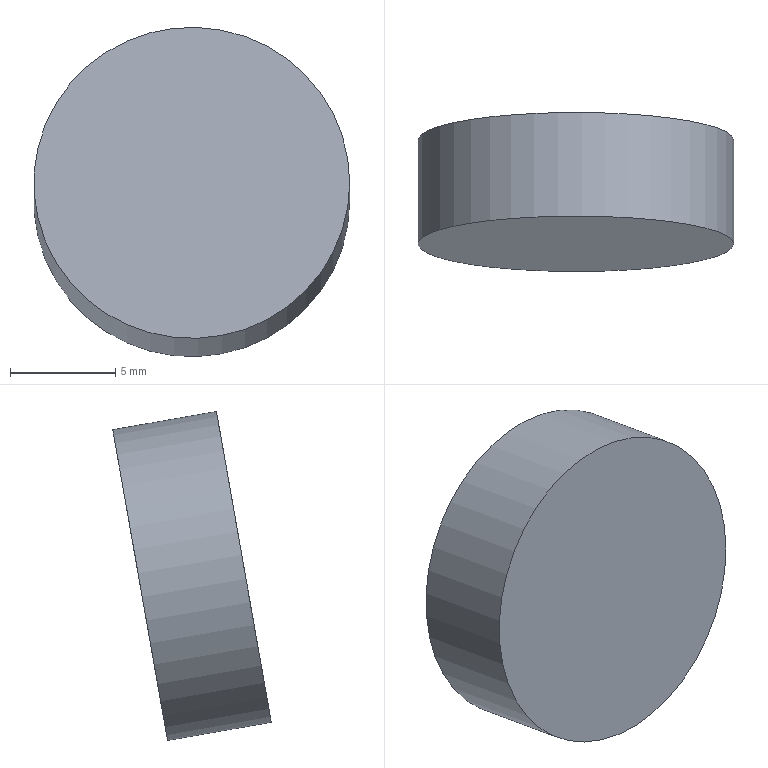Part | NX | features solid 2 | 1 solid | 3 faces | box 15 x 7.529 x 15.64 mm | volume 883.573 mm3 | plane 2 | cylinder 1 | commonest cylinder face diameters 15 x1
STEP:
#1=CARTESIAN_POINT('',(-1001.,-834.668,49.225));
#2=VERTEX_POINT('',#1);
#3=CARTESIAN_POINT('',(-1008.5,-834.668,49.225));
#4=DIRECTION('',(0.,-0.9848,0.1736));
#5=DIRECTION('',(1.,0.,0.));
#6=AXIS2_PLACEMENT_3D('',#3,#4,#5);
#7=CIRCLE('',#6,7.5);
#8=EDGE_CURVE('',#2,#2,#7,.T.);
#9=ORIENTED_EDGE('',*,*,#8,.T.);
#10=EDGE_LOOP('',(#9));
#11=FACE_BOUND('',#10,.T.);
#12=CARTESIAN_POINT('',(-1001.,-839.592,50.093));
#13=VERTEX_POINT('',#12);
#14=CARTESIAN_POINT('',(-1008.5,-839.592,50.093));
#15=DIRECTION('',(0.,-0.9848,0.1736));
#16=DIRECTION('',(1.,0.,0.));
#17=AXIS2_PLACEMENT_3D('',#14,#15,#16);
#18=CIRCLE('',#17,7.5);
#19=EDGE_CURVE('',#13,#13,#18,.T.);
#20=ORIENTED_EDGE('',*,*,#19,.F.);
#21=EDGE_LOOP('',(#20));
#22=FACE_BOUND('',#21,.T.);
#23=CARTESIAN_POINT('',(-1008.5,-839.592,50.093));
#24=DIRECTION('',(0.,0.9848,-0.1736));
#25=DIRECTION('',(-1.,0.,0.));
#26=AXIS2_PLACEMENT_3D('',#23,#24,#25);
#27=CYLINDRICAL_SURFACE('',#26,7.5);
#28=ADVANCED_FACE('',(#11,#22),#27,.T.);
#29=ORIENTED_EDGE('',*,*,#19,.T.);
#30=EDGE_LOOP('',(#29));
#31=FACE_BOUND('',#30,.T.);
#32=CARTESIAN_POINT('',(-1008.5,-839.592,50.093));
#33=DIRECTION('',(0.,-0.9848,0.1736));
#34=DIRECTION('',(1.,0.,0.));
#35=AXIS2_PLACEMENT_3D('',#32,#33,#34);
#36=PLANE('',#35);
#37=ADVANCED_FACE('',(#31),#36,.T.);
#38=ORIENTED_EDGE('',*,*,#8,.F.);
#39=EDGE_LOOP('',(#38));
#40=FACE_BOUND('',#39,.T.);
#41=CARTESIAN_POINT('',(-1008.5,-834.668,49.225));
#42=DIRECTION('',(0.,-0.9848,0.1736));
#43=DIRECTION('',(0.,-0.1736,-0.9848));
#44=AXIS2_PLACEMENT_3D('',#41,#42,#43);
#45=PLANE('',#44);
#46=ADVANCED_FACE('',(#40),#45,.F.);
#47=CLOSED_SHELL('',(#28,#37,#46));
#48=MANIFOLD_SOLID_BREP('',#47);
#49=(LENGTH_UNIT()NAMED_UNIT(*)SI_UNIT(.MILLI.,.METRE.));
#50=UNCERTAINTY_MEASURE_WITH_UNIT(LENGTH_MEASURE(0.00001),#49,'','');
#51=(NAMED_UNIT(*)PLANE_ANGLE_UNIT()SI_UNIT($,.RADIAN.));
#52=(NAMED_UNIT(*)SI_UNIT($,.STERADIAN.)SOLID_ANGLE_UNIT());
#53=(GEOMETRIC_REPRESENTATION_CONTEXT(3)GLOBAL_UNCERTAINTY_ASSIGNED_CONTEXT((#50))GLOBAL_UNIT_ASSIGNED_CONTEXT((#49,#51,#52))REPRESENTATION_CONTEXT('',''));
#54=ADVANCED_BREP_SHAPE_REPRESENTATION('',(#48),#53);